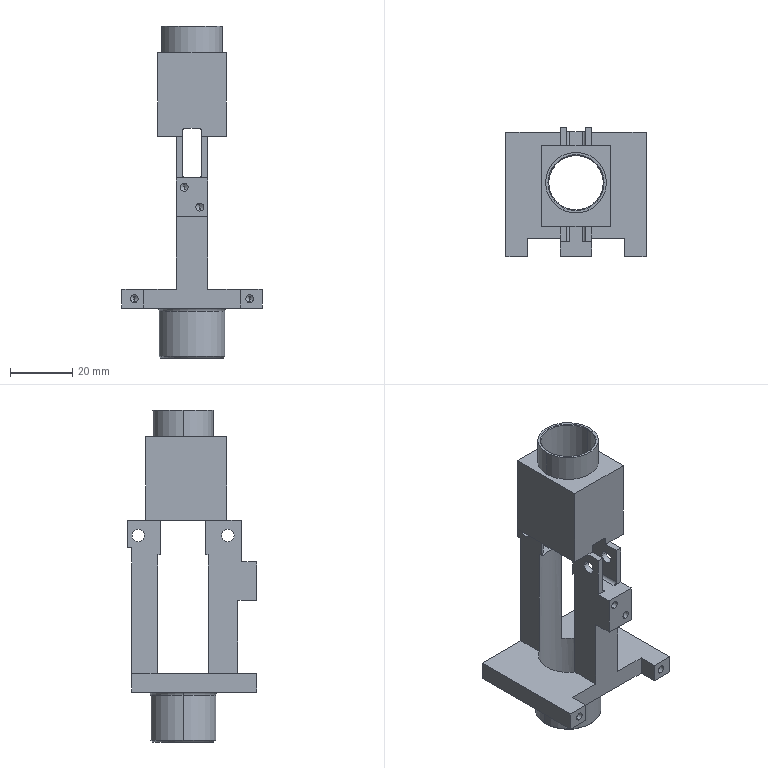Part | SolidWorks | features ICE 25, Chamfer 5, HoleWzd 5, Fillet 2, Attribute 1, CenterOfMass 1, Extrusion 1 | 1 solid | 110 faces | box 45 x 41.44 x 106.5 mm | volume 25458 mm3 | plane 48 | cylinder 40 | cone 20 | torus 2 | commonest cylinder face diameters 2.5 x16 2 x8 4.02 x4 4.06 x4 17.5 x2 19 x2